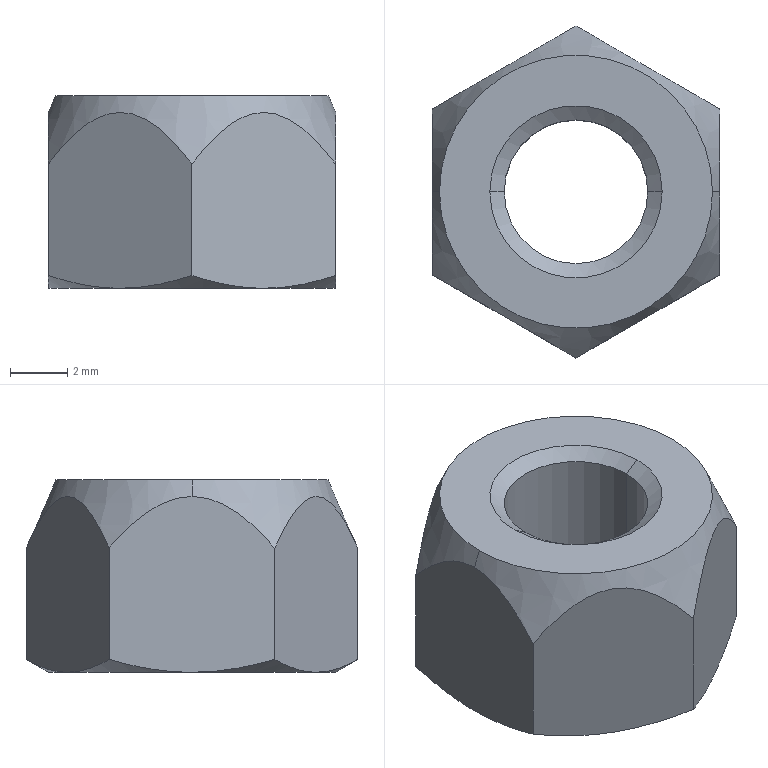Part | STEP file | prevailing torque hex nut_am_AM-M6-N | 1 solid | 24 faces | box 10 x 11.547 x 6.7 mm | volume 433.135 mm3 | cone 12 | plane 8 | cylinder 4 | commonest cylinder face diameters 5 x2 6 x2